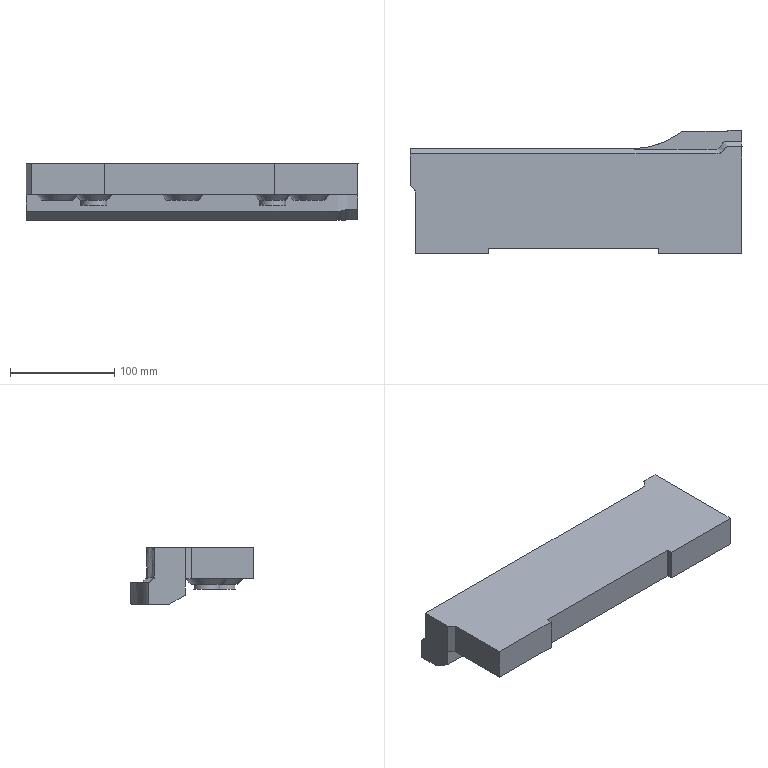Part | NX | features solid 2 | 1 solid | 34 faces | box 317.88 x 118.2 x 54.615 mm | volume 1185553 mm3 | plane 19 | spline 8 | cone 5 | cylinder 2 | commonest cylinder face diameters 25 x2